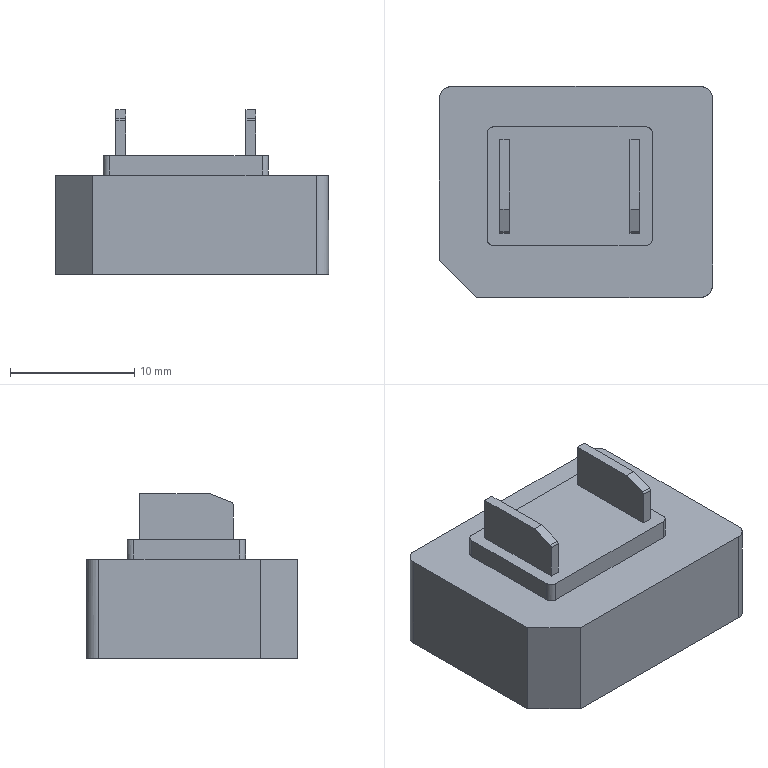CAM job | PowerMill | 3-axis milling, other | part box 22 x 17 x 13.286 mm
Tools:
number,name,type,diameter,tip_radius,length,cutting_length,overhang,flutes,holder,toolpaths_using
1,D10C,end_mill,10.0,0.0,60.0,,30.0,1,D42L35,1
1,D10C_1_1,end_mill,10.0,0.0,60.0,,13.72,1,D42L35,3
2,D4C_1_1,end_mill,4.0,0.0,30.0,,5.44,1,D42L35,1
3,D10_1_1,end_mill,10.0,0.0,60.0,,13.44,1,D42L35,4
4,R1_1_1,ball_nosed,2.0,1.0,3.0,,2.16,1,D42L35,1
10,D3_1_1,end_mill,3.0,0.0,30.0,,4.04,1,D42L35,2
13,Text_D4_1_1,taper_spherical,4.0,0.3,60.0,,5.56,1,D42L35,1
Operations:
program,toolpath,strategy,tool,tool_number,tool_diameter,tip_radius,flutes,spindle_rpm,feed_cut,surface_speed_m_min_computed,feed_per_tooth_computed,tolerance,thickness,stepover,stepdown,cut_length,cut_time_min,total_time_min,workplane
006-0625-3-F,精公开粗01-扫面平行-D10C,raster_area_clear,D10C_1_1,1,10.0,0.0,1.0,8000.0,10000.0,251.33,1.25,0.03,0.3,6.0,1.0,160.6,0.016,0.0205,
006-0625-3-F,精公开粗01-外形偏置-D10C,offset_area_clear,D10C_1_1,1,10.0,0.0,1.0,8000.0,10000.0,251.33,1.25,0.03,0.3,6.0,1.0,2641.097,0.264,0.3006,
006-0625-3-F,精公开粗01-基准台等高-D10C,constantz,D10C_1_1,1,10.0,0.0,1.0,8000.0,10000.0,251.33,1.25,0.03,0.07,5.0,0.4,2349.114,0.235,0.2432,
006-0625-3-F,精公再粗02-外形偏置-D4C,offset_area_clear,D4C_1_1,2,4.0,0.0,1.0,18000.0,6000.0,226.19,0.3333,0.03,0.02,2.0,1.0,1979.913,0.33,0.4243,
006-0625-3-F,精公基准台01-平坦面偏置-D10,offset_area_clear,D10_1_1,3,10.0,0.0,1.0,8500.0,600.0,267.04,0.0706,0.005,0.4,5.0,1.0,124.28,0.207,0.238,
006-0625-3-F,精公基准台01-基准面偏置-D10,offset_area_clear,D10_1_1,3,10.0,0.0,1.0,8500.0,600.0,267.04,0.0706,0.005,0.4,5.0,1.0,88.152,0.147,0.1641,
006-0625-3-F,精公基准台01-外形侧光-D10,profile_area_clear,D10_1_1,3,10.0,0.0,1.0,8500.0,600.0,267.04,0.0706,0.005,-0.05,0.08,1.0,152.342,0.254,0.273,
006-0625-3-F,精公基准台01-基准台侧光-D10,profile_area_clear,D10_1_1,3,10.0,0.0,1.0,8500.0,600.0,267.04,0.0706,0.005,0.0,0.08,1.0,213.233,0.355,0.4181,
006-0625-3-F,精公精光01-平行-R1,raster,R1_1_1,4,2.0,1.0,1.0,18000.0,2000.0,113.1,0.1111,0.005,-0.055,0.03,1.0,244.837,0.122,0.133,
006-0625-3-F,精公精光02-等高-D3,constantz,D3_1_1,10,3.0,0.0,1.0,18000.0,2000.0,169.65,0.1111,0.005,-0.055,5.0,0.03,6268.903,3.135,3.444,
006-0625-3-F,精公精光02-平坦面偏置-D3,offset_area_clear,D3_1_1,10,3.0,0.0,1.0,18000.0,600.0,169.65,0.0333,0.005,0.395,1.5,1.0,128.975,0.215,0.2497,
006-0625-3-F,精公刻字01-刻字-Text_D4,pattern,Text_D4_1_1,13,4.0,0.3,1.0,15000.0,1000.0,188.5,0.0667,0.005,0.0,5.0,1.0,35.384,0.035,0.0518,
,精公开粗01-外形偏置-D10C_Reference,offset_area_clear,D10C,1,10.0,0.0,1.0,8000.0,10000.0,251.33,1.25,0.03,0.3,6.0,1.0,5089.905,0.509,0.5771,